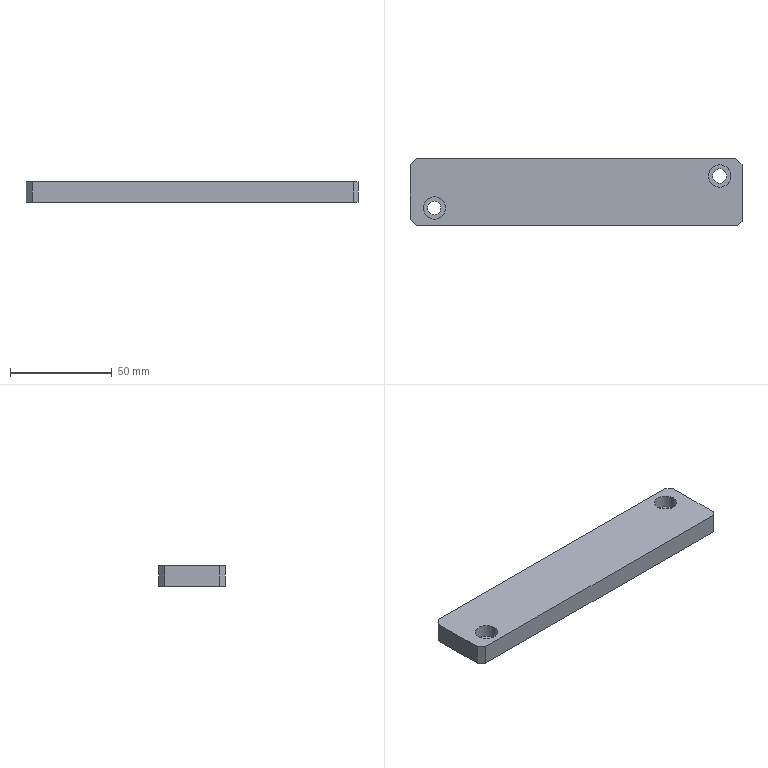Part | STEP file | 1_id534_x_t | 1 solid | 29 faces | box 163.45 x 32.752 x 10 mm | volume 50026 mm3 | plane 15 | cylinder 14 | commonest cylinder face diameters 12 x6 11 x4 6.5 x2 7 x2